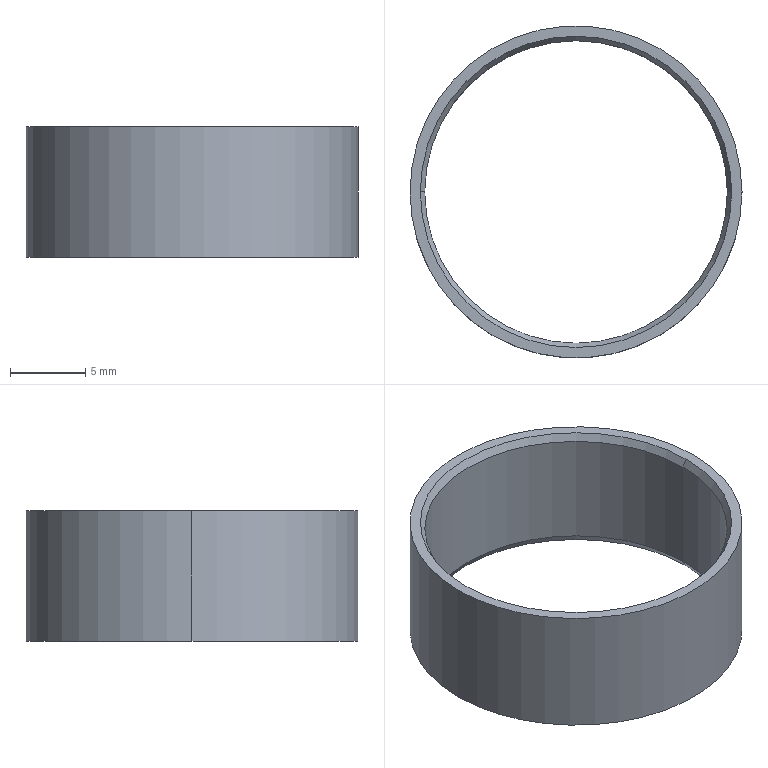Part | SolidWorks | features Chamfer 1, Extrusion 1 | 1 solid | 10 faces | box 22 x 22 x 8.66 mm | volume 548.531 mm3 | cone 4 | cylinder 4 | plane 2 | commonest cylinder face diameters 20.05 x2 22 x2
STEP:
#1=CARTESIAN_POINT('',(10.025,0.,0.5));
#2=VERTEX_POINT('',#1);
#3=CARTESIAN_POINT('',(-10.025,0.,0.5));
#4=VERTEX_POINT('',#3);
#5=CARTESIAN_POINT('',(0.,0.,0.5));
#6=DIRECTION('',(0.,0.,-1.));
#7=DIRECTION('',(1.,0.,0.));
#8=AXIS2_PLACEMENT_3D('',#5,#6,#7);
#9=CIRCLE('',#8,10.025);
#10=EDGE_CURVE('',#2,#4,#9,.T.);
#11=ORIENTED_EDGE('',*,*,#10,.F.);
#12=CARTESIAN_POINT('',(10.314,0.,0.));
#13=VERTEX_POINT('',#12);
#14=CARTESIAN_POINT('',(10.314,0.,0.));
#15=DIRECTION('',(0.5,0.,-0.866));
#16=VECTOR('',#15,1000.);
#17=LINE('',#14,#16);
#18=EDGE_CURVE('',#2,#13,#17,.T.);
#19=ORIENTED_EDGE('',*,*,#18,.T.);
#20=CARTESIAN_POINT('',(-10.314,0.,0.));
#21=VERTEX_POINT('',#20);
#22=CARTESIAN_POINT('',(0.,0.,0.));
#23=DIRECTION('',(0.,0.,1.));
#24=DIRECTION('',(1.,0.,0.));
#25=AXIS2_PLACEMENT_3D('',#22,#23,#24);
#26=CIRCLE('',#25,10.314);
#27=EDGE_CURVE('',#21,#13,#26,.T.);
#28=ORIENTED_EDGE('',*,*,#27,.F.);
#29=CARTESIAN_POINT('',(-10.314,0.,0.));
#30=DIRECTION('',(-0.5,0.,-0.866));
#31=VECTOR('',#30,1000.);
#32=LINE('',#29,#31);
#33=EDGE_CURVE('',#4,#21,#32,.T.);
#34=ORIENTED_EDGE('',*,*,#33,.F.);
#35=EDGE_LOOP('',(#11,#19,#28,#34));
#36=FACE_OUTER_BOUND('',#35,.T.);
#37=CARTESIAN_POINT('',(0.,0.,0.));
#38=DIRECTION('',(0.,0.,-1.));
#39=DIRECTION('',(-1.,0.,0.));
#40=AXIS2_PLACEMENT_3D('',#37,#38,#39);
#41=CONICAL_SURFACE('',#40,10.314,0.5236);
#42=ADVANCED_FACE('',(#36),#41,.F.);
#43=CARTESIAN_POINT('',(-10.025,0.,8.16));
#44=VERTEX_POINT('',#43);
#45=CARTESIAN_POINT('',(10.025,0.,8.16));
#46=VERTEX_POINT('',#45);
#47=CARTESIAN_POINT('',(0.,0.,8.16));
#48=DIRECTION('',(0.,0.,1.));
#49=DIRECTION('',(1.,0.,0.));
#50=AXIS2_PLACEMENT_3D('',#47,#48,#49);
#51=CIRCLE('',#50,10.025);
#52=EDGE_CURVE('',#44,#46,#51,.T.);
#53=ORIENTED_EDGE('',*,*,#52,.F.);
#54=CARTESIAN_POINT('',(-10.314,0.,8.66));
#55=VERTEX_POINT('',#54);
#56=CARTESIAN_POINT('',(-10.025,0.,8.16));
#57=DIRECTION('',(-0.5,0.,0.866));
#58=VECTOR('',#57,1000.);
#59=LINE('',#56,#58);
#60=EDGE_CURVE('',#44,#55,#59,.T.);
#61=ORIENTED_EDGE('',*,*,#60,.T.);
#62=CARTESIAN_POINT('',(10.314,0.,8.66));
#63=VERTEX_POINT('',#62);
#64=CARTESIAN_POINT('',(0.,0.,8.66));
#65=DIRECTION('',(0.,0.,-1.));
#66=DIRECTION('',(1.,0.,0.));
#67=AXIS2_PLACEMENT_3D('',#64,#65,#66);
#68=CIRCLE('',#67,10.314);
#69=EDGE_CURVE('',#63,#55,#68,.T.);
#70=ORIENTED_EDGE('',*,*,#69,.F.);
#71=CARTESIAN_POINT('',(10.025,0.,8.16));
#72=DIRECTION('',(0.5,0.,0.866));
#73=VECTOR('',#72,1000.);
#74=LINE('',#71,#73);
#75=EDGE_CURVE('',#46,#63,#74,.T.);
#76=ORIENTED_EDGE('',*,*,#75,.F.);
#77=EDGE_LOOP('',(#53,#61,#70,#76));
#78=FACE_OUTER_BOUND('',#77,.T.);
#79=CARTESIAN_POINT('',(0.,0.,8.16));
#80=DIRECTION('',(0.,0.,1.));
#81=DIRECTION('',(1.,0.,0.));
#82=AXIS2_PLACEMENT_3D('',#79,#80,#81);
#83=CONICAL_SURFACE('',#82,10.025,0.5236);
#84=ADVANCED_FACE('',(#78),#83,.F.);
#85=ORIENTED_EDGE('',*,*,#52,.T.);
#86=CARTESIAN_POINT('',(10.025,0.,8.66));
#87=DIRECTION('',(0.,0.,-1.));
#88=VECTOR('',#87,1000.);
#89=LINE('',#86,#88);
#90=EDGE_CURVE('',#46,#2,#89,.T.);
#91=ORIENTED_EDGE('',*,*,#90,.T.);
#92=ORIENTED_EDGE('',*,*,#10,.T.);
#93=CARTESIAN_POINT('',(-10.025,0.,8.66));
#94=DIRECTION('',(0.,0.,-1.));
#95=VECTOR('',#94,1000.);
#96=LINE('',#93,#95);
#97=EDGE_CURVE('',#44,#4,#96,.T.);
#98=ORIENTED_EDGE('',*,*,#97,.F.);
#99=EDGE_LOOP('',(#85,#91,#92,#98));
#100=FACE_OUTER_BOUND('',#99,.T.);
#101=CARTESIAN_POINT('',(0.,0.,8.66));
#102=DIRECTION('',(0.,0.,-1.));
#103=DIRECTION('',(-1.,0.,0.));
#104=AXIS2_PLACEMENT_3D('',#101,#102,#103);
#105=CYLINDRICAL_SURFACE('',#104,10.025);
#106=ADVANCED_FACE('',(#100),#105,.F.);
#107=CARTESIAN_POINT('',(11.,0.,8.66));
#108=VERTEX_POINT('',#107);
#109=CARTESIAN_POINT('',(-11.,0.,8.66));
#110=VERTEX_POINT('',#109);
#111=CARTESIAN_POINT('',(0.,0.,8.66));
#112=DIRECTION('',(0.,0.,1.));
#113=DIRECTION('',(1.,0.,0.));
#114=AXIS2_PLACEMENT_3D('',#111,#112,#113);
#115=CIRCLE('',#114,11.);
#116=EDGE_CURVE('',#108,#110,#115,.T.);
#117=ORIENTED_EDGE('',*,*,#116,.F.);
#118=CARTESIAN_POINT('',(11.,0.,0.));
#119=VERTEX_POINT('',#118);
#120=CARTESIAN_POINT('',(11.,0.,8.66));
#121=DIRECTION('',(0.,0.,-1.));
#122=VECTOR('',#121,1000.);
#123=LINE('',#120,#122);
#124=EDGE_CURVE('',#108,#119,#123,.T.);
#125=ORIENTED_EDGE('',*,*,#124,.T.);
#126=CARTESIAN_POINT('',(-11.,0.,0.));
#127=VERTEX_POINT('',#126);
#128=CARTESIAN_POINT('',(0.,0.,0.));
#129=DIRECTION('',(0.,0.,1.));
#130=DIRECTION('',(1.,0.,0.));
#131=AXIS2_PLACEMENT_3D('',#128,#129,#130);
#132=CIRCLE('',#131,11.);
#133=EDGE_CURVE('',#119,#127,#132,.T.);
#134=ORIENTED_EDGE('',*,*,#133,.T.);
#135=CARTESIAN_POINT('',(-11.,0.,8.66));
#136=DIRECTION('',(0.,0.,-1.));
#137=VECTOR('',#136,1000.);
#138=LINE('',#135,#137);
#139=EDGE_CURVE('',#110,#127,#138,.T.);
#140=ORIENTED_EDGE('',*,*,#139,.F.);
#141=EDGE_LOOP('',(#117,#125,#134,#140));
#142=FACE_OUTER_BOUND('',#141,.T.);
#143=CARTESIAN_POINT('',(0.,0.,8.66));
#144=DIRECTION('',(0.,0.,-1.));
#145=DIRECTION('',(-1.,0.,0.));
#146=AXIS2_PLACEMENT_3D('',#143,#144,#145);
#147=CYLINDRICAL_SURFACE('',#146,11.);
#148=ADVANCED_FACE('',(#142),#147,.T.);
#149=ORIENTED_EDGE('',*,*,#69,.T.);
#150=CARTESIAN_POINT('',(0.,0.,8.66));
#151=DIRECTION('',(0.,0.,-1.));
#152=DIRECTION('',(1.,0.,0.));
#153=AXIS2_PLACEMENT_3D('',#150,#151,#152);
#154=CIRCLE('',#153,10.314);
#155=EDGE_CURVE('',#55,#63,#154,.T.);
#156=ORIENTED_EDGE('',*,*,#155,.T.);
#157=EDGE_LOOP('',(#149,#156));
#158=FACE_BOUND('',#157,.T.);
#159=CARTESIAN_POINT('',(0.,0.,8.66));
#160=DIRECTION('',(0.,0.,1.));
#161=DIRECTION('',(1.,0.,0.));
#162=AXIS2_PLACEMENT_3D('',#159,#160,#161);
#163=CIRCLE('',#162,11.);
#164=EDGE_CURVE('',#110,#108,#163,.T.);
#165=ORIENTED_EDGE('',*,*,#164,.T.);
#166=ORIENTED_EDGE('',*,*,#116,.T.);
#167=EDGE_LOOP('',(#165,#166));
#168=FACE_OUTER_BOUND('',#167,.T.);
#169=CARTESIAN_POINT('',(0.,0.,8.66));
#170=DIRECTION('',(0.,0.,1.));
#171=DIRECTION('',(1.,0.,0.));
#172=AXIS2_PLACEMENT_3D('',#169,#170,#171);
#173=PLANE('',#172);
#174=ADVANCED_FACE('',(#158,#168),#173,.T.);
#175=ORIENTED_EDGE('',*,*,#27,.T.);
#176=CARTESIAN_POINT('',(0.,0.,0.));
#177=DIRECTION('',(0.,0.,1.));
#178=DIRECTION('',(1.,0.,0.));
#179=AXIS2_PLACEMENT_3D('',#176,#177,#178);
#180=CIRCLE('',#179,10.314);
#181=EDGE_CURVE('',#13,#21,#180,.T.);
#182=ORIENTED_EDGE('',*,*,#181,.T.);
#183=EDGE_LOOP('',(#175,#182));
#184=FACE_BOUND('',#183,.T.);
#185=CARTESIAN_POINT('',(0.,0.,0.));
#186=DIRECTION('',(0.,0.,1.));
#187=DIRECTION('',(1.,0.,0.));
#188=AXIS2_PLACEMENT_3D('',#185,#186,#187);
#189=CIRCLE('',#188,11.);
#190=EDGE_CURVE('',#127,#119,#189,.T.);
#191=ORIENTED_EDGE('',*,*,#190,.F.);
#192=ORIENTED_EDGE('',*,*,#133,.F.);
#193=EDGE_LOOP('',(#191,#192));
#194=FACE_OUTER_BOUND('',#193,.T.);
#195=CARTESIAN_POINT('',(0.,0.,0.));
#196=DIRECTION('',(0.,0.,1.));
#197=DIRECTION('',(1.,0.,0.));
#198=AXIS2_PLACEMENT_3D('',#195,#196,#197);
#199=PLANE('',#198);
#200=ADVANCED_FACE('',(#184,#194),#199,.F.);
#201=ORIENTED_EDGE('',*,*,#124,.F.);
#202=ORIENTED_EDGE('',*,*,#164,.F.);
#203=ORIENTED_EDGE('',*,*,#139,.T.);
#204=ORIENTED_EDGE('',*,*,#190,.T.);
#205=EDGE_LOOP('',(#201,#202,#203,#204));
#206=FACE_OUTER_BOUND('',#205,.T.);
#207=CARTESIAN_POINT('',(0.,0.,8.66));
#208=DIRECTION('',(0.,0.,-1.));
#209=DIRECTION('',(-1.,0.,0.));
#210=AXIS2_PLACEMENT_3D('',#207,#208,#209);
#211=CYLINDRICAL_SURFACE('',#210,11.);
#212=ADVANCED_FACE('',(#206),#211,.T.);
#213=ORIENTED_EDGE('',*,*,#90,.F.);
#214=CARTESIAN_POINT('',(0.,0.,8.16));
#215=DIRECTION('',(0.,0.,1.));
#216=DIRECTION('',(1.,0.,0.));
#217=AXIS2_PLACEMENT_3D('',#214,#215,#216);
#218=CIRCLE('',#217,10.025);
#219=EDGE_CURVE('',#46,#44,#218,.T.);
#220=ORIENTED_EDGE('',*,*,#219,.T.);
#221=ORIENTED_EDGE('',*,*,#97,.T.);
#222=CARTESIAN_POINT('',(0.,0.,0.5));
#223=DIRECTION('',(0.,0.,-1.));
#224=DIRECTION('',(1.,0.,0.));
#225=AXIS2_PLACEMENT_3D('',#222,#223,#224);
#226=CIRCLE('',#225,10.025);
#227=EDGE_CURVE('',#4,#2,#226,.T.);
#228=ORIENTED_EDGE('',*,*,#227,.T.);
#229=EDGE_LOOP('',(#213,#220,#221,#228));
#230=FACE_OUTER_BOUND('',#229,.T.);
#231=CARTESIAN_POINT('',(0.,0.,8.66));
#232=DIRECTION('',(0.,0.,-1.));
#233=DIRECTION('',(-1.,0.,0.));
#234=AXIS2_PLACEMENT_3D('',#231,#232,#233);
#235=CYLINDRICAL_SURFACE('',#234,10.025);
#236=ADVANCED_FACE('',(#230),#235,.F.);
#237=ORIENTED_EDGE('',*,*,#60,.F.);
#238=ORIENTED_EDGE('',*,*,#219,.F.);
#239=ORIENTED_EDGE('',*,*,#75,.T.);
#240=ORIENTED_EDGE('',*,*,#155,.F.);
#241=EDGE_LOOP('',(#237,#238,#239,#240));
#242=FACE_OUTER_BOUND('',#241,.T.);
#243=CARTESIAN_POINT('',(0.,0.,8.16));
#244=DIRECTION('',(0.,0.,1.));
#245=DIRECTION('',(1.,0.,0.));
#246=AXIS2_PLACEMENT_3D('',#243,#244,#245);
#247=CONICAL_SURFACE('',#246,10.025,0.5236);
#248=ADVANCED_FACE('',(#242),#247,.F.);
#249=ORIENTED_EDGE('',*,*,#18,.F.);
#250=ORIENTED_EDGE('',*,*,#227,.F.);
#251=ORIENTED_EDGE('',*,*,#33,.T.);
#252=ORIENTED_EDGE('',*,*,#181,.F.);
#253=EDGE_LOOP('',(#249,#250,#251,#252));
#254=FACE_OUTER_BOUND('',#253,.T.);
#255=CARTESIAN_POINT('',(0.,0.,0.));
#256=DIRECTION('',(0.,0.,-1.));
#257=DIRECTION('',(-1.,0.,0.));
#258=AXIS2_PLACEMENT_3D('',#255,#256,#257);
#259=CONICAL_SURFACE('',#258,10.314,0.5236);
#260=ADVANCED_FACE('',(#254),#259,.F.);
#261=CLOSED_SHELL('',(#42,#84,#106,#148,#174,#200,#212,#236,#248,#260));
#262=MANIFOLD_SOLID_BREP('',#261);
#263=CARTESIAN_POINT('',(0.,0.,0.));
#264=DIRECTION('',(0.,0.,1.));
#265=DIRECTION('',(1.,0.,0.));
#266=AXIS2_PLACEMENT_3D('',#263,#264,#265);
#267=(LENGTH_UNIT()NAMED_UNIT(*)SI_UNIT(.MILLI.,.METRE.));
#268=UNCERTAINTY_MEASURE_WITH_UNIT(LENGTH_MEASURE(0.00001),#267,'','');
#269=(NAMED_UNIT(*)PLANE_ANGLE_UNIT()SI_UNIT($,.RADIAN.));
#270=(NAMED_UNIT(*)SI_UNIT($,.STERADIAN.)SOLID_ANGLE_UNIT());
#271=(GEOMETRIC_REPRESENTATION_CONTEXT(3)GLOBAL_UNCERTAINTY_ASSIGNED_CONTEXT((#268))GLOBAL_UNIT_ASSIGNED_CONTEXT((#267,#269,#270))REPRESENTATION_CONTEXT('',''));
#272=ADVANCED_BREP_SHAPE_REPRESENTATION('',(#262,#266),#271);